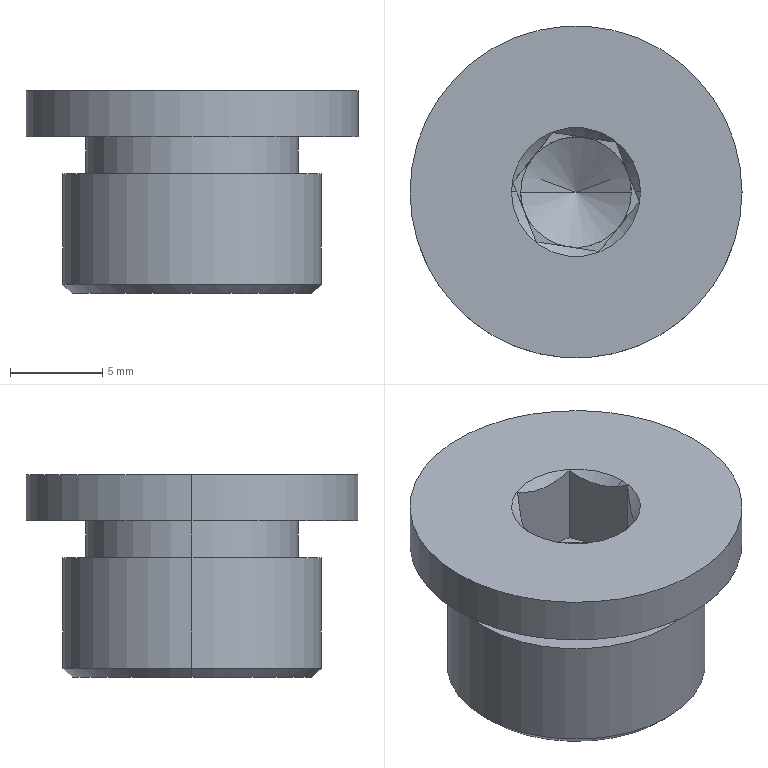Part | SolidWorks | features BaseBody 1 | 1 solid | 30 faces | box 18 x 18 x 11 mm | volume 1653 mm3 | plane 16 | cylinder 8 | cone 6 | commonest cylinder face diameters 6 x2 11.5 x2 14 x2 18 x2
STEP:
#1=CARTESIAN_POINT('',(-10.901,8.92,75.5));
#2=VERTEX_POINT('',#1);
#3=CARTESIAN_POINT('',(-28.901,8.92,75.5));
#4=VERTEX_POINT('',#3);
#5=CARTESIAN_POINT('',(-19.901,8.92,75.5));
#6=DIRECTION('',(0.,0.,1.));
#7=DIRECTION('',(1.,0.,0.));
#8=AXIS2_PLACEMENT_3D('',#5,#6,#7);
#9=CIRCLE('',#8,9.);
#10=EDGE_CURVE('',#2,#4,#9,.T.);
#11=ORIENTED_EDGE('',*,*,#10,.T.);
#12=CARTESIAN_POINT('',(-28.901,8.92,78.));
#13=VERTEX_POINT('',#12);
#14=CARTESIAN_POINT('',(-28.901,8.92,75.5));
#15=DIRECTION('',(0.,0.,1.));
#16=VECTOR('',#15,1000.);
#17=LINE('',#14,#16);
#18=EDGE_CURVE('',#4,#13,#17,.T.);
#19=ORIENTED_EDGE('',*,*,#18,.T.);
#20=CARTESIAN_POINT('',(-10.901,8.92,78.));
#21=VERTEX_POINT('',#20);
#22=CARTESIAN_POINT('',(-19.901,8.92,78.));
#23=DIRECTION('',(0.,0.,1.));
#24=DIRECTION('',(1.,0.,0.));
#25=AXIS2_PLACEMENT_3D('',#22,#23,#24);
#26=CIRCLE('',#25,9.);
#27=EDGE_CURVE('',#21,#13,#26,.T.);
#28=ORIENTED_EDGE('',*,*,#27,.F.);
#29=CARTESIAN_POINT('',(-10.901,8.92,75.5));
#30=DIRECTION('',(0.,0.,1.));
#31=VECTOR('',#30,1000.);
#32=LINE('',#29,#31);
#33=EDGE_CURVE('',#2,#21,#32,.T.);
#34=ORIENTED_EDGE('',*,*,#33,.F.);
#35=EDGE_LOOP('',(#11,#19,#28,#34));
#36=FACE_OUTER_BOUND('',#35,.T.);
#37=CARTESIAN_POINT('',(-19.901,8.92,75.5));
#38=DIRECTION('',(0.,0.,1.));
#39=DIRECTION('',(1.,0.,0.));
#40=AXIS2_PLACEMENT_3D('',#37,#38,#39);
#41=CYLINDRICAL_SURFACE('',#40,9.);
#42=ADVANCED_FACE('',(#36),#41,.T.);
#43=CARTESIAN_POINT('',(-14.151,8.92,73.5));
#44=VERTEX_POINT('',#43);
#45=CARTESIAN_POINT('',(-25.651,8.92,73.5));
#46=VERTEX_POINT('',#45);
#47=CARTESIAN_POINT('',(-19.901,8.92,73.5));
#48=DIRECTION('',(0.,0.,1.));
#49=DIRECTION('',(1.,0.,0.));
#50=AXIS2_PLACEMENT_3D('',#47,#48,#49);
#51=CIRCLE('',#50,5.75);
#52=EDGE_CURVE('',#44,#46,#51,.T.);
#53=ORIENTED_EDGE('',*,*,#52,.T.);
#54=CARTESIAN_POINT('',(-25.651,8.92,75.5));
#55=VERTEX_POINT('',#54);
#56=CARTESIAN_POINT('',(-25.651,8.92,73.5));
#57=DIRECTION('',(0.,0.,1.));
#58=VECTOR('',#57,1000.);
#59=LINE('',#56,#58);
#60=EDGE_CURVE('',#46,#55,#59,.T.);
#61=ORIENTED_EDGE('',*,*,#60,.T.);
#62=CARTESIAN_POINT('',(-14.151,8.92,75.5));
#63=VERTEX_POINT('',#62);
#64=CARTESIAN_POINT('',(-19.901,8.92,75.5));
#65=DIRECTION('',(0.,0.,-1.));
#66=DIRECTION('',(1.,0.,0.));
#67=AXIS2_PLACEMENT_3D('',#64,#65,#66);
#68=CIRCLE('',#67,5.75);
#69=EDGE_CURVE('',#55,#63,#68,.T.);
#70=ORIENTED_EDGE('',*,*,#69,.T.);
#71=CARTESIAN_POINT('',(-14.151,8.92,73.5));
#72=DIRECTION('',(0.,0.,1.));
#73=VECTOR('',#72,1000.);
#74=LINE('',#71,#73);
#75=EDGE_CURVE('',#44,#63,#74,.T.);
#76=ORIENTED_EDGE('',*,*,#75,.F.);
#77=EDGE_LOOP('',(#53,#61,#70,#76));
#78=FACE_OUTER_BOUND('',#77,.T.);
#79=CARTESIAN_POINT('',(-19.901,8.92,73.5));
#80=DIRECTION('',(0.,0.,1.));
#81=DIRECTION('',(1.,0.,0.));
#82=AXIS2_PLACEMENT_3D('',#79,#80,#81);
#83=CYLINDRICAL_SURFACE('',#82,5.75);
#84=ADVANCED_FACE('',(#78),#83,.T.);
#85=CARTESIAN_POINT('',(-22.901,8.92,72.5));
#86=VERTEX_POINT('',#85);
#87=CARTESIAN_POINT('',(-16.901,8.92,72.5));
#88=VERTEX_POINT('',#87);
#89=CARTESIAN_POINT('',(-19.901,8.92,72.5));
#90=DIRECTION('',(0.,0.,1.));
#91=DIRECTION('',(1.,0.,0.));
#92=AXIS2_PLACEMENT_3D('',#89,#90,#91);
#93=CIRCLE('',#92,3.);
#94=EDGE_CURVE('',#86,#88,#93,.T.);
#95=ORIENTED_EDGE('',*,*,#94,.F.);
#96=CARTESIAN_POINT('',(-22.901,8.92,73.5));
#97=VERTEX_POINT('',#96);
#98=CARTESIAN_POINT('',(-22.901,8.92,72.5));
#99=DIRECTION('',(0.,0.,1.));
#100=VECTOR('',#99,1000.);
#101=LINE('',#98,#100);
#102=EDGE_CURVE('',#86,#97,#101,.T.);
#103=ORIENTED_EDGE('',*,*,#102,.T.);
#104=CARTESIAN_POINT('',(-22.698,7.835,73.5));
#105=VERTEX_POINT('',#104);
#106=CARTESIAN_POINT('',(-19.901,8.92,73.5));
#107=DIRECTION('',(0.,0.,-1.));
#108=DIRECTION('',(1.,0.,0.));
#109=AXIS2_PLACEMENT_3D('',#106,#107,#108);
#110=CIRCLE('',#109,3.);
#111=EDGE_CURVE('',#105,#97,#110,.T.);
#112=ORIENTED_EDGE('',*,*,#111,.F.);
#113=CARTESIAN_POINT('',(-20.36,5.955,73.5));
#114=VERTEX_POINT('',#113);
#115=CARTESIAN_POINT('',(-19.901,8.92,73.5));
#116=DIRECTION('',(0.,0.,-1.));
#117=DIRECTION('',(1.,0.,0.));
#118=AXIS2_PLACEMENT_3D('',#115,#116,#117);
#119=CIRCLE('',#118,3.);
#120=EDGE_CURVE('',#114,#105,#119,.T.);
#121=ORIENTED_EDGE('',*,*,#120,.F.);
#122=CARTESIAN_POINT('',(-17.563,7.04,73.5));
#123=VERTEX_POINT('',#122);
#124=CARTESIAN_POINT('',(-19.901,8.92,73.5));
#125=DIRECTION('',(0.,0.,-1.));
#126=DIRECTION('',(1.,0.,0.));
#127=AXIS2_PLACEMENT_3D('',#124,#125,#126);
#128=CIRCLE('',#127,3.);
#129=EDGE_CURVE('',#123,#114,#128,.T.);
#130=ORIENTED_EDGE('',*,*,#129,.F.);
#131=CARTESIAN_POINT('',(-16.901,8.92,73.5));
#132=VERTEX_POINT('',#131);
#133=CARTESIAN_POINT('',(-19.901,8.92,73.5));
#134=DIRECTION('',(0.,0.,-1.));
#135=DIRECTION('',(1.,0.,0.));
#136=AXIS2_PLACEMENT_3D('',#133,#134,#135);
#137=CIRCLE('',#136,3.);
#138=EDGE_CURVE('',#132,#123,#137,.T.);
#139=ORIENTED_EDGE('',*,*,#138,.F.);
#140=CARTESIAN_POINT('',(-16.901,8.92,72.5));
#141=DIRECTION('',(0.,0.,1.));
#142=VECTOR('',#141,1000.);
#143=LINE('',#140,#142);
#144=EDGE_CURVE('',#88,#132,#143,.T.);
#145=ORIENTED_EDGE('',*,*,#144,.F.);
#146=EDGE_LOOP('',(#95,#103,#112,#121,#130,#139,#145));
#147=FACE_OUTER_BOUND('',#146,.T.);
#148=CARTESIAN_POINT('',(-19.901,8.92,72.5));
#149=DIRECTION('',(0.,0.,1.));
#150=DIRECTION('',(1.,0.,0.));
#151=AXIS2_PLACEMENT_3D('',#148,#149,#150);
#152=CYLINDRICAL_SURFACE('',#151,3.);
#153=ADVANCED_FACE('',(#147),#152,.F.);
#154=CARTESIAN_POINT('',(-19.901,8.92,70.768));
#155=VERTEX_POINT('',#154);
#156=CARTESIAN_POINT('',(-16.901,8.92,72.5));
#157=DIRECTION('',(0.866,0.,0.5));
#158=VECTOR('',#157,1000.);
#159=LINE('',#156,#158);
#160=EDGE_CURVE('',#155,#88,#159,.T.);
#161=ORIENTED_EDGE('',*,*,#160,.F.);
#162=CARTESIAN_POINT('',(-22.901,8.92,72.5));
#163=DIRECTION('',(-0.866,0.,0.5));
#164=VECTOR('',#163,1000.);
#165=LINE('',#162,#164);
#166=EDGE_CURVE('',#155,#86,#165,.T.);
#167=ORIENTED_EDGE('',*,*,#166,.T.);
#168=ORIENTED_EDGE('',*,*,#94,.T.);
#169=EDGE_LOOP('',(#161,#167,#168));
#170=FACE_OUTER_BOUND('',#169,.T.);
#171=CARTESIAN_POINT('',(-19.901,8.92,72.5));
#172=DIRECTION('',(0.,0.,1.));
#173=DIRECTION('',(1.,0.,0.));
#174=AXIS2_PLACEMENT_3D('',#171,#172,#173);
#175=CONICAL_SURFACE('',#174,3.,1.047);
#176=ADVANCED_FACE('',(#170),#175,.F.);
#177=CARTESIAN_POINT('',(-12.901,8.92,67.5));
#178=VERTEX_POINT('',#177);
#179=CARTESIAN_POINT('',(-26.901,8.92,67.5));
#180=VERTEX_POINT('',#179);
#181=CARTESIAN_POINT('',(-19.901,8.92,67.5));
#182=DIRECTION('',(0.,0.,1.));
#183=DIRECTION('',(1.,0.,0.));
#184=AXIS2_PLACEMENT_3D('',#181,#182,#183);
#185=CIRCLE('',#184,7.);
#186=EDGE_CURVE('',#178,#180,#185,.T.);
#187=ORIENTED_EDGE('',*,*,#186,.T.);
#188=CARTESIAN_POINT('',(-26.901,8.92,73.5));
#189=VERTEX_POINT('',#188);
#190=CARTESIAN_POINT('',(-26.901,8.92,67.5));
#191=DIRECTION('',(0.,0.,1.));
#192=VECTOR('',#191,1000.);
#193=LINE('',#190,#192);
#194=EDGE_CURVE('',#180,#189,#193,.T.);
#195=ORIENTED_EDGE('',*,*,#194,.T.);
#196=CARTESIAN_POINT('',(-12.901,8.92,73.5));
#197=VERTEX_POINT('',#196);
#198=CARTESIAN_POINT('',(-19.901,8.92,73.5));
#199=DIRECTION('',(0.,0.,1.));
#200=DIRECTION('',(1.,0.,0.));
#201=AXIS2_PLACEMENT_3D('',#198,#199,#200);
#202=CIRCLE('',#201,7.);
#203=EDGE_CURVE('',#197,#189,#202,.T.);
#204=ORIENTED_EDGE('',*,*,#203,.F.);
#205=CARTESIAN_POINT('',(-12.901,8.92,67.5));
#206=DIRECTION('',(0.,0.,1.));
#207=VECTOR('',#206,1000.);
#208=LINE('',#205,#207);
#209=EDGE_CURVE('',#178,#197,#208,.T.);
#210=ORIENTED_EDGE('',*,*,#209,.F.);
#211=EDGE_LOOP('',(#187,#195,#204,#210));
#212=FACE_OUTER_BOUND('',#211,.T.);
#213=CARTESIAN_POINT('',(-19.901,8.92,67.5));
#214=DIRECTION('',(0.,0.,1.));
#215=DIRECTION('',(1.,0.,0.));
#216=AXIS2_PLACEMENT_3D('',#213,#214,#215);
#217=CYLINDRICAL_SURFACE('',#216,7.);
#218=ADVANCED_FACE('',(#212),#217,.T.);
#219=CARTESIAN_POINT('',(-13.401,8.92,67.));
#220=VERTEX_POINT('',#219);
#221=CARTESIAN_POINT('',(-26.401,8.92,67.));
#222=VERTEX_POINT('',#221);
#223=CARTESIAN_POINT('',(-19.901,8.92,67.));
#224=DIRECTION('',(0.,0.,1.));
#225=DIRECTION('',(1.,0.,0.));
#226=AXIS2_PLACEMENT_3D('',#223,#224,#225);
#227=CIRCLE('',#226,6.5);
#228=EDGE_CURVE('',#220,#222,#227,.T.);
#229=ORIENTED_EDGE('',*,*,#228,.T.);
#230=CARTESIAN_POINT('',(-26.901,8.92,67.5));
#231=DIRECTION('',(-0.7071,0.,0.7071));
#232=VECTOR('',#231,1000.);
#233=LINE('',#230,#232);
#234=EDGE_CURVE('',#222,#180,#233,.T.);
#235=ORIENTED_EDGE('',*,*,#234,.T.);
#236=ORIENTED_EDGE('',*,*,#186,.F.);
#237=CARTESIAN_POINT('',(-12.901,8.92,67.5));
#238=DIRECTION('',(0.7071,0.,0.7071));
#239=VECTOR('',#238,1000.);
#240=LINE('',#237,#239);
#241=EDGE_CURVE('',#220,#178,#240,.T.);
#242=ORIENTED_EDGE('',*,*,#241,.F.);
#243=EDGE_LOOP('',(#229,#235,#236,#242));
#244=FACE_OUTER_BOUND('',#243,.T.);
#245=CARTESIAN_POINT('',(-19.901,8.92,67.5));
#246=DIRECTION('',(0.,0.,1.));
#247=DIRECTION('',(1.,0.,0.));
#248=AXIS2_PLACEMENT_3D('',#245,#246,#247);
#249=CONICAL_SURFACE('',#248,7.,0.7854);
#250=ADVANCED_FACE('',(#244),#249,.T.);
#251=CARTESIAN_POINT('',(-16.401,8.92,78.));
#252=VERTEX_POINT('',#251);
#253=CARTESIAN_POINT('',(-23.401,8.92,78.));
#254=VERTEX_POINT('',#253);
#255=CARTESIAN_POINT('',(-19.901,8.92,78.));
#256=DIRECTION('',(0.,0.,-1.));
#257=DIRECTION('',(1.,0.,0.));
#258=AXIS2_PLACEMENT_3D('',#255,#256,#257);
#259=CIRCLE('',#258,3.5);
#260=EDGE_CURVE('',#252,#254,#259,.T.);
#261=ORIENTED_EDGE('',*,*,#260,.T.);
#262=CARTESIAN_POINT('',(-19.901,8.92,78.));
#263=DIRECTION('',(0.,0.,-1.));
#264=DIRECTION('',(1.,0.,0.));
#265=AXIS2_PLACEMENT_3D('',#262,#263,#264);
#266=CIRCLE('',#265,3.5);
#267=EDGE_CURVE('',#254,#252,#266,.T.);
#268=ORIENTED_EDGE('',*,*,#267,.T.);
#269=EDGE_LOOP('',(#261,#268));
#270=FACE_BOUND('',#269,.T.);
#271=ORIENTED_EDGE('',*,*,#27,.T.);
#272=CARTESIAN_POINT('',(-19.901,8.92,78.));
#273=DIRECTION('',(0.,0.,1.));
#274=DIRECTION('',(1.,0.,0.));
#275=AXIS2_PLACEMENT_3D('',#272,#273,#274);
#276=CIRCLE('',#275,9.);
#277=EDGE_CURVE('',#13,#21,#276,.T.);
#278=ORIENTED_EDGE('',*,*,#277,.T.);
#279=EDGE_LOOP('',(#271,#278));
#280=FACE_OUTER_BOUND('',#279,.T.);
#281=CARTESIAN_POINT('',(-19.901,8.92,78.));
#282=DIRECTION('',(0.,0.,1.));
#283=DIRECTION('',(1.,0.,0.));
#284=AXIS2_PLACEMENT_3D('',#281,#282,#283);
#285=PLANE('',#284);
#286=ADVANCED_FACE('',(#270,#280),#285,.T.);
#287=CARTESIAN_POINT('',(-23.325,9.449,77.964));
#288=VERTEX_POINT('',#287);
#289=CARTESIAN_POINT('',(-23.119,8.92,77.718));
#290=VERTEX_POINT('',#289);
#291=CARTESIAN_POINT('',(-23.325,9.449,77.964));
#292=CARTESIAN_POINT('',(-23.258,9.277,77.872));
#293=CARTESIAN_POINT('',(-23.189,9.101,77.788));
#294=CARTESIAN_POINT('',(-23.119,8.92,77.718));
#295=B_SPLINE_CURVE_WITH_KNOTS('',3,(#291,#292,#293,#294),.UNSPECIFIED.,.F.,.F.,(4,4),(0.,0.0006191),.UNSPECIFIED.);
#296=EDGE_CURVE('',#288,#290,#295,.T.);
#297=ORIENTED_EDGE('',*,*,#296,.F.);
#298=CARTESIAN_POINT('',(-21.154,12.149,77.964));
#299=VERTEX_POINT('',#298);
#300=CARTESIAN_POINT('',(-21.154,12.149,77.964));
#301=CARTESIAN_POINT('',(-21.324,11.938,77.829));
#302=CARTESIAN_POINT('',(-21.497,11.723,77.714));
#303=CARTESIAN_POINT('',(-21.767,11.388,77.59));
#304=CARTESIAN_POINT('',(-21.858,11.274,77.558));
#305=CARTESIAN_POINT('',(-22.045,11.042,77.512));
#306=CARTESIAN_POINT('',(-22.141,10.922,77.5));
#307=CARTESIAN_POINT('',(-22.425,10.569,77.499));
#308=CARTESIAN_POINT('',(-22.611,10.337,77.545));
#309=CARTESIAN_POINT('',(-22.978,9.88,77.711));
#310=CARTESIAN_POINT('',(-23.154,9.662,77.828));
#311=CARTESIAN_POINT('',(-23.325,9.449,77.964));
#312=B_SPLINE_CURVE_WITH_KNOTS('',3,(#300,#301,#302,#303,#304,#305,#306,#307,#308,#309,#310,#311),.UNSPECIFIED.,.F.,.F.,(4,2,2,2,2,4),(0.,0.0008946,0.001342,0.001789,0.002684,0.003578),.UNSPECIFIED.);
#313=EDGE_CURVE('',#299,#288,#312,.T.);
#314=ORIENTED_EDGE('',*,*,#313,.F.);
#315=CARTESIAN_POINT('',(-17.731,11.62,77.964));
#316=VERTEX_POINT('',#315);
#317=CARTESIAN_POINT('',(-17.731,11.62,77.964));
#318=CARTESIAN_POINT('',(-17.998,11.661,77.829));
#319=CARTESIAN_POINT('',(-18.272,11.703,77.714));
#320=CARTESIAN_POINT('',(-18.697,11.769,77.59));
#321=CARTESIAN_POINT('',(-18.841,11.791,77.558));
#322=CARTESIAN_POINT('',(-19.135,11.837,77.512));
#323=CARTESIAN_POINT('',(-19.287,11.86,77.5));
#324=CARTESIAN_POINT('',(-19.735,11.93,77.499));
#325=CARTESIAN_POINT('',(-20.029,11.975,77.545));
#326=CARTESIAN_POINT('',(-20.608,12.065,77.711));
#327=CARTESIAN_POINT('',(-20.885,12.108,77.828));
#328=CARTESIAN_POINT('',(-21.154,12.149,77.964));
#329=B_SPLINE_CURVE_WITH_KNOTS('',3,(#317,#318,#319,#320,#321,#322,#323,#324,#325,#326,#327,#328),.UNSPECIFIED.,.F.,.F.,(4,2,2,2,2,4),(0.,0.0008946,0.001342,0.001789,0.002684,0.003578),.UNSPECIFIED.);
#330=EDGE_CURVE('',#316,#299,#329,.T.);
#331=ORIENTED_EDGE('',*,*,#330,.F.);
#332=CARTESIAN_POINT('',(-16.683,8.92,77.718));
#333=VERTEX_POINT('',#332);
#334=CARTESIAN_POINT('',(-16.683,8.92,77.718));
#335=CARTESIAN_POINT('',(-16.769,9.14,77.632));
#336=CARTESIAN_POINT('',(-16.856,9.365,77.568));
#337=CARTESIAN_POINT('',(-17.034,9.823,77.496));
#338=CARTESIAN_POINT('',(-17.126,10.061,77.49));
#339=CARTESIAN_POINT('',(-17.395,10.755,77.566));
#340=CARTESIAN_POINT('',(-17.568,11.2,77.739));
#341=CARTESIAN_POINT('',(-17.731,11.62,77.964));
#342=B_SPLINE_CURVE_WITH_KNOTS('',3,(#334,#335,#336,#337,#338,#339,#340,#341),.UNSPECIFIED.,.F.,.F.,(4,2,2,4),(0.,0.0007448,0.00149,0.002979),.UNSPECIFIED.);
#343=EDGE_CURVE('',#333,#316,#342,.T.);
#344=ORIENTED_EDGE('',*,*,#343,.F.);
#345=CARTESIAN_POINT('',(-16.401,8.92,78.));
#346=CARTESIAN_POINT('',(-16.683,8.92,77.718));
#347=B_SPLINE_CURVE_WITH_KNOTS('',1,(#345,#346),.UNSPECIFIED.,.F.,.F.,(2,2),(0.,1.),.UNSPECIFIED.);
#348=EDGE_CURVE('',#252,#333,#347,.T.);
#349=ORIENTED_EDGE('',*,*,#348,.F.);
#350=ORIENTED_EDGE('',*,*,#267,.F.);
#351=CARTESIAN_POINT('',(-23.119,8.92,77.718));
#352=CARTESIAN_POINT('',(-23.401,8.92,78.));
#353=B_SPLINE_CURVE_WITH_KNOTS('',1,(#351,#352),.UNSPECIFIED.,.F.,.F.,(2,2),(0.,1.),.UNSPECIFIED.);
#354=EDGE_CURVE('',#290,#254,#353,.T.);
#355=ORIENTED_EDGE('',*,*,#354,.F.);
#356=EDGE_LOOP('',(#297,#314,#331,#344,#349,#350,#355));
#357=FACE_OUTER_BOUND('',#356,.T.);
#358=CARTESIAN_POINT('',(-19.901,8.92,78.));
#359=DIRECTION('',(0.,0.,1.));
#360=DIRECTION('',(1.,0.,0.));
#361=AXIS2_PLACEMENT_3D('',#358,#359,#360);
#362=CONICAL_SURFACE('',#361,3.5,0.7854);
#363=ADVANCED_FACE('',(#357),#362,.F.);
#364=ORIENTED_EDGE('',*,*,#354,.T.);
#365=ORIENTED_EDGE('',*,*,#260,.F.);
#366=ORIENTED_EDGE('',*,*,#348,.T.);
#367=CARTESIAN_POINT('',(-16.478,8.39,77.964));
#368=VERTEX_POINT('',#367);
#369=CARTESIAN_POINT('',(-16.478,8.39,77.964));
#370=CARTESIAN_POINT('',(-16.545,8.563,77.872));
#371=CARTESIAN_POINT('',(-16.613,8.739,77.788));
#372=CARTESIAN_POINT('',(-16.683,8.92,77.718));
#373=B_SPLINE_CURVE_WITH_KNOTS('',3,(#369,#370,#371,#372),.UNSPECIFIED.,.F.,.F.,(4,4),(0.,0.0006191),.UNSPECIFIED.);
#374=EDGE_CURVE('',#368,#333,#373,.T.);
#375=ORIENTED_EDGE('',*,*,#374,.F.);
#376=CARTESIAN_POINT('',(-18.648,5.69,77.964));
#377=VERTEX_POINT('',#376);
#378=CARTESIAN_POINT('',(-18.648,5.69,77.964));
#379=CARTESIAN_POINT('',(-18.479,5.901,77.829));
#380=CARTESIAN_POINT('',(-18.305,6.117,77.714));
#381=CARTESIAN_POINT('',(-18.036,6.452,77.59));
#382=CARTESIAN_POINT('',(-17.944,6.566,77.558));
#383=CARTESIAN_POINT('',(-17.758,6.798,77.512));
#384=CARTESIAN_POINT('',(-17.662,6.917,77.5));
#385=CARTESIAN_POINT('',(-17.378,7.271,77.499));
#386=CARTESIAN_POINT('',(-17.191,7.503,77.545));
#387=CARTESIAN_POINT('',(-16.824,7.96,77.711));
#388=CARTESIAN_POINT('',(-16.648,8.178,77.828));
#389=CARTESIAN_POINT('',(-16.478,8.39,77.964));
#390=B_SPLINE_CURVE_WITH_KNOTS('',3,(#378,#379,#380,#381,#382,#383,#384,#385,#386,#387,#388,#389),.UNSPECIFIED.,.F.,.F.,(4,2,2,2,2,4),(0.,0.0008946,0.001342,0.001789,0.002684,0.003578),.UNSPECIFIED.);
#391=EDGE_CURVE('',#377,#368,#390,.T.);
#392=ORIENTED_EDGE('',*,*,#391,.F.);
#393=CARTESIAN_POINT('',(-22.072,6.22,77.964));
#394=VERTEX_POINT('',#393);
#395=CARTESIAN_POINT('',(-22.072,6.22,77.964));
#396=CARTESIAN_POINT('',(-21.804,6.179,77.829));
#397=CARTESIAN_POINT('',(-21.531,6.136,77.714));
#398=CARTESIAN_POINT('',(-21.106,6.07,77.59));
#399=CARTESIAN_POINT('',(-20.962,6.048,77.558));
#400=CARTESIAN_POINT('',(-20.667,6.003,77.512));
#401=CARTESIAN_POINT('',(-20.516,5.979,77.5));
#402=CARTESIAN_POINT('',(-20.067,5.91,77.499));
#403=CARTESIAN_POINT('',(-19.774,5.864,77.545));
#404=CARTESIAN_POINT('',(-19.194,5.775,77.711));
#405=CARTESIAN_POINT('',(-18.917,5.732,77.828));
#406=CARTESIAN_POINT('',(-18.648,5.69,77.964));
#407=B_SPLINE_CURVE_WITH_KNOTS('',3,(#395,#396,#397,#398,#399,#400,#401,#402,#403,#404,#405,#406),.UNSPECIFIED.,.F.,.F.,(4,2,2,2,2,4),(0.,0.0008946,0.001342,0.001789,0.002684,0.003578),.UNSPECIFIED.);
#408=EDGE_CURVE('',#394,#377,#407,.T.);
#409=ORIENTED_EDGE('',*,*,#408,.F.);
#410=CARTESIAN_POINT('',(-23.119,8.92,77.718));
#411=CARTESIAN_POINT('',(-23.034,8.699,77.632));
#412=CARTESIAN_POINT('',(-22.947,8.475,77.568));
#413=CARTESIAN_POINT('',(-22.769,8.017,77.496));
#414=CARTESIAN_POINT('',(-22.676,7.779,77.49));
#415=CARTESIAN_POINT('',(-22.407,7.085,77.566));
#416=CARTESIAN_POINT('',(-22.234,6.639,77.739));
#417=CARTESIAN_POINT('',(-22.072,6.22,77.964));
#418=B_SPLINE_CURVE_WITH_KNOTS('',3,(#410,#411,#412,#413,#414,#415,#416,#417),.UNSPECIFIED.,.F.,.F.,(4,2,2,4),(0.,0.0007448,0.00149,0.002979),.UNSPECIFIED.);
#419=EDGE_CURVE('',#290,#394,#418,.T.);
#420=ORIENTED_EDGE('',*,*,#419,.F.);
#421=EDGE_LOOP('',(#364,#365,#366,#375,#392,#409,#420));
#422=FACE_OUTER_BOUND('',#421,.T.);
#423=CARTESIAN_POINT('',(-19.901,8.92,78.));
#424=DIRECTION('',(0.,0.,1.));
#425=DIRECTION('',(1.,0.,0.));
#426=AXIS2_PLACEMENT_3D('',#423,#424,#425);
#427=CONICAL_SURFACE('',#426,3.5,0.7854);
#428=ADVANCED_FACE('',(#422),#427,.F.);
#429=ORIENTED_EDGE('',*,*,#18,.F.);
#430=CARTESIAN_POINT('',(-19.901,8.92,75.5));
#431=DIRECTION('',(0.,0.,1.));
#432=DIRECTION('',(1.,0.,0.));
#433=AXIS2_PLACEMENT_3D('',#430,#431,#432);
#434=CIRCLE('',#433,9.);
#435=EDGE_CURVE('',#4,#2,#434,.T.);
#436=ORIENTED_EDGE('',*,*,#435,.T.);
#437=ORIENTED_EDGE('',*,*,#33,.T.);
#438=ORIENTED_EDGE('',*,*,#277,.F.);
#439=EDGE_LOOP('',(#429,#436,#437,#438));
#440=FACE_OUTER_BOUND('',#439,.T.);
#441=CARTESIAN_POINT('',(-19.901,8.92,75.5));
#442=DIRECTION('',(0.,0.,1.));
#443=DIRECTION('',(1.,0.,0.));
#444=AXIS2_PLACEMENT_3D('',#441,#442,#443);
#445=CYLINDRICAL_SURFACE('',#444,9.);
#446=ADVANCED_FACE('',(#440),#445,.T.);
#447=ORIENTED_EDGE('',*,*,#313,.T.);
#448=CARTESIAN_POINT('',(-23.325,9.449,73.5));
#449=VERTEX_POINT('',#448);
#450=CARTESIAN_POINT('',(-23.325,9.449,75.732));
#451=DIRECTION('',(0.,0.,-1.));
#452=VECTOR('',#451,1000.);
#453=LINE('',#450,#452);
#454=EDGE_CURVE('',#288,#449,#453,.T.);
#455=ORIENTED_EDGE('',*,*,#454,.T.);
#456=CARTESIAN_POINT('',(-22.239,10.799,73.5));
#457=VERTEX_POINT('',#456);
#458=CARTESIAN_POINT('',(-22.239,10.799,73.5));
#459=DIRECTION('',(-0.6265,-0.7794,0.));
#460=VECTOR('',#459,1000.);
#461=LINE('',#458,#460);
#462=EDGE_CURVE('',#457,#449,#461,.T.);
#463=ORIENTED_EDGE('',*,*,#462,.F.);
#464=CARTESIAN_POINT('',(-21.154,12.149,73.5));
#465=VERTEX_POINT('',#464);
#466=CARTESIAN_POINT('',(-21.154,12.149,73.5));
#467=DIRECTION('',(-0.6265,-0.7794,0.));
#468=VECTOR('',#467,1000.);
#469=LINE('',#466,#468);
#470=EDGE_CURVE('',#465,#457,#469,.T.);
#471=ORIENTED_EDGE('',*,*,#470,.F.);
#472=CARTESIAN_POINT('',(-21.154,12.149,75.732));
#473=DIRECTION('',(0.,0.,1.));
#474=VECTOR('',#473,1000.);
#475=LINE('',#472,#474);
#476=EDGE_CURVE('',#465,#299,#475,.T.);
#477=ORIENTED_EDGE('',*,*,#476,.T.);
#478=EDGE_LOOP('',(#447,#455,#463,#471,#477));
#479=FACE_OUTER_BOUND('',#478,.T.);
#480=CARTESIAN_POINT('',(-22.239,10.799,75.732));
#481=DIRECTION('',(0.7794,-0.6265,0.));
#482=DIRECTION('',(0.6265,0.7794,0.));
#483=AXIS2_PLACEMENT_3D('',#480,#481,#482);
#484=PLANE('',#483);
#485=ADVANCED_FACE('',(#479),#484,.T.);
#486=CARTESIAN_POINT('',(-17.731,11.62,73.5));
#487=VERTEX_POINT('',#486);
#488=CARTESIAN_POINT('',(-19.443,11.885,73.5));
#489=VERTEX_POINT('',#488);
#490=CARTESIAN_POINT('',(-17.731,11.62,73.5));
#491=DIRECTION('',(-0.9882,0.1529,0.));
#492=VECTOR('',#491,1000.);
#493=LINE('',#490,#492);
#494=EDGE_CURVE('',#487,#489,#493,.T.);
#495=ORIENTED_EDGE('',*,*,#494,.F.);
#496=CARTESIAN_POINT('',(-17.731,11.62,75.732));
#497=DIRECTION('',(0.,0.,-1.));
#498=VECTOR('',#497,1000.);
#499=LINE('',#496,#498);
#500=EDGE_CURVE('',#316,#487,#499,.T.);
#501=ORIENTED_EDGE('',*,*,#500,.F.);
#502=ORIENTED_EDGE('',*,*,#330,.T.);
#503=ORIENTED_EDGE('',*,*,#476,.F.);
#504=CARTESIAN_POINT('',(-19.443,11.885,73.5));
#505=DIRECTION('',(-0.9882,0.1529,0.));
#506=VECTOR('',#505,1000.);
#507=LINE('',#504,#506);
#508=EDGE_CURVE('',#489,#465,#507,.T.);
#509=ORIENTED_EDGE('',*,*,#508,.F.);
#510=EDGE_LOOP('',(#495,#501,#502,#503,#509));
#511=FACE_OUTER_BOUND('',#510,.T.);
#512=CARTESIAN_POINT('',(-19.443,11.885,75.732));
#513=DIRECTION('',(0.1529,0.9882,0.));
#514=DIRECTION('',(-0.9882,0.1529,0.));
#515=AXIS2_PLACEMENT_3D('',#512,#513,#514);
#516=PLANE('',#515);
#517=ADVANCED_FACE('',(#511),#516,.F.);
#518=CARTESIAN_POINT('',(-16.478,8.39,73.5));
#519=VERTEX_POINT('',#518);
#520=CARTESIAN_POINT('',(-17.104,10.005,73.5));
#521=VERTEX_POINT('',#520);
#522=CARTESIAN_POINT('',(-16.478,8.39,73.5));
#523=DIRECTION('',(-0.3617,0.9323,0.));
#524=VECTOR('',#523,1000.);
#525=LINE('',#522,#524);
#526=EDGE_CURVE('',#519,#521,#525,.T.);
#527=ORIENTED_EDGE('',*,*,#526,.F.);
#528=CARTESIAN_POINT('',(-16.478,8.39,75.732));
#529=DIRECTION('',(0.,0.,-1.));
#530=VECTOR('',#529,1000.);
#531=LINE('',#528,#530);
#532=EDGE_CURVE('',#368,#519,#531,.T.);
#533=ORIENTED_EDGE('',*,*,#532,.F.);
#534=ORIENTED_EDGE('',*,*,#374,.T.);
#535=ORIENTED_EDGE('',*,*,#343,.T.);
#536=ORIENTED_EDGE('',*,*,#500,.T.);
#537=CARTESIAN_POINT('',(-17.104,10.005,73.5));
#538=DIRECTION('',(-0.3617,0.9323,0.));
#539=VECTOR('',#538,1000.);
#540=LINE('',#537,#539);
#541=EDGE_CURVE('',#521,#487,#540,.T.);
#542=ORIENTED_EDGE('',*,*,#541,.F.);
#543=EDGE_LOOP('',(#527,#533,#534,#535,#536,#542));
#544=FACE_OUTER_BOUND('',#543,.T.);
#545=CARTESIAN_POINT('',(-17.104,10.005,75.732));
#546=DIRECTION('',(0.9323,0.3617,0.));
#547=DIRECTION('',(-0.3617,0.9323,0.));
#548=AXIS2_PLACEMENT_3D('',#545,#546,#547);
#549=PLANE('',#548);
#550=ADVANCED_FACE('',(#544),#549,.F.);
#551=ORIENTED_EDGE('',*,*,#419,.T.);
#552=CARTESIAN_POINT('',(-22.072,6.22,73.5));
#553=VERTEX_POINT('',#552);
#554=CARTESIAN_POINT('',(-22.072,6.22,75.732));
#555=DIRECTION('',(0.,0.,-1.));
#556=VECTOR('',#555,1000.);
#557=LINE('',#554,#556);
#558=EDGE_CURVE('',#394,#553,#557,.T.);
#559=ORIENTED_EDGE('',*,*,#558,.T.);
#560=CARTESIAN_POINT('',(-22.698,7.835,73.5));
#561=DIRECTION('',(0.3617,-0.9323,0.));
#562=VECTOR('',#561,1000.);
#563=LINE('',#560,#562);
#564=EDGE_CURVE('',#105,#553,#563,.T.);
#565=ORIENTED_EDGE('',*,*,#564,.F.);
#566=CARTESIAN_POINT('',(-23.325,9.449,73.5));
#567=DIRECTION('',(0.3617,-0.9323,0.));
#568=VECTOR('',#567,1000.);
#569=LINE('',#566,#568);
#570=EDGE_CURVE('',#449,#105,#569,.T.);
#571=ORIENTED_EDGE('',*,*,#570,.F.);
#572=ORIENTED_EDGE('',*,*,#454,.F.);
#573=ORIENTED_EDGE('',*,*,#296,.T.);
#574=EDGE_LOOP('',(#551,#559,#565,#571,#572,#573));
#575=FACE_OUTER_BOUND('',#574,.T.);
#576=CARTESIAN_POINT('',(-22.698,7.835,75.732));
#577=DIRECTION('',(0.9323,0.3617,0.));
#578=DIRECTION('',(-0.3617,0.9323,0.));
#579=AXIS2_PLACEMENT_3D('',#576,#577,#578);
#580=PLANE('',#579);
#581=ADVANCED_FACE('',(#575),#580,.T.);
#582=CARTESIAN_POINT('',(-17.563,7.04,73.5));
#583=DIRECTION('',(0.6265,0.7794,0.));
#584=VECTOR('',#583,1000.);
#585=LINE('',#582,#584);
#586=EDGE_CURVE('',#123,#519,#585,.T.);
#587=ORIENTED_EDGE('',*,*,#586,.F.);
#588=CARTESIAN_POINT('',(-18.648,5.69,73.5));
#589=VERTEX_POINT('',#588);
#590=CARTESIAN_POINT('',(-18.648,5.69,73.5));
#591=DIRECTION('',(0.6265,0.7794,0.));
#592=VECTOR('',#591,1000.);
#593=LINE('',#590,#592);
#594=EDGE_CURVE('',#589,#123,#593,.T.);
#595=ORIENTED_EDGE('',*,*,#594,.F.);
#596=CARTESIAN_POINT('',(-18.648,5.69,75.732));
#597=DIRECTION('',(0.,0.,-1.));
#598=VECTOR('',#597,1000.);
#599=LINE('',#596,#598);
#600=EDGE_CURVE('',#377,#589,#599,.T.);
#601=ORIENTED_EDGE('',*,*,#600,.F.);
#602=ORIENTED_EDGE('',*,*,#391,.T.);
#603=ORIENTED_EDGE('',*,*,#532,.T.);
#604=EDGE_LOOP('',(#587,#595,#601,#602,#603));
#605=FACE_OUTER_BOUND('',#604,.T.);
#606=CARTESIAN_POINT('',(-17.563,7.04,75.732));
#607=DIRECTION('',(0.7794,-0.6265,0.));
#608=DIRECTION('',(0.6265,0.7794,0.));
#609=AXIS2_PLACEMENT_3D('',#606,#607,#608);
#610=PLANE('',#609);
#611=ADVANCED_FACE('',(#605),#610,.F.);
#612=ORIENTED_EDGE('',*,*,#408,.T.);
#613=ORIENTED_EDGE('',*,*,#600,.T.);
#614=CARTESIAN_POINT('',(-20.36,5.955,73.5));
#615=DIRECTION('',(0.9882,-0.1529,0.));
#616=VECTOR('',#615,1000.);
#617=LINE('',#614,#616);
#618=EDGE_CURVE('',#114,#589,#617,.T.);
#619=ORIENTED_EDGE('',*,*,#618,.F.);
#620=CARTESIAN_POINT('',(-20.36,5.955,73.5));
#621=DIRECTION('',(-0.9882,0.1529,0.));
#622=VECTOR('',#621,1000.);
#623=LINE('',#620,#622);
#624=EDGE_CURVE('',#114,#553,#623,.T.);
#625=ORIENTED_EDGE('',*,*,#624,.T.);
#626=ORIENTED_EDGE('',*,*,#558,.F.);
#627=EDGE_LOOP('',(#612,#613,#619,#625,#626));
#628=FACE_OUTER_BOUND('',#627,.T.);
#629=CARTESIAN_POINT('',(-20.36,5.955,75.732));
#630=DIRECTION('',(0.1529,0.9882,0.));
#631=DIRECTION('',(-0.9882,0.1529,0.));
#632=AXIS2_PLACEMENT_3D('',#629,#630,#631);
#633=PLANE('',#632);
#634=ADVANCED_FACE('',(#628),#633,.T.);
#635=CARTESIAN_POINT('',(-19.901,8.92,75.5));
#636=DIRECTION('',(0.,0.,-1.));
#637=DIRECTION('',(1.,0.,0.));
#638=AXIS2_PLACEMENT_3D('',#635,#636,#637);
#639=CIRCLE('',#638,5.75);
#640=EDGE_CURVE('',#63,#55,#639,.T.);
#641=ORIENTED_EDGE('',*,*,#640,.F.);
#642=ORIENTED_EDGE('',*,*,#69,.F.);
#643=EDGE_LOOP('',(#641,#642));
#644=FACE_BOUND('',#643,.T.);
#645=ORIENTED_EDGE('',*,*,#10,.F.);
#646=ORIENTED_EDGE('',*,*,#435,.F.);
#647=EDGE_LOOP('',(#645,#646));
#648=FACE_OUTER_BOUND('',#647,.T.);
#649=CARTESIAN_POINT('',(-19.901,8.92,75.5));
#650=DIRECTION('',(0.,0.,1.));
#651=DIRECTION('',(1.,0.,0.));
#652=AXIS2_PLACEMENT_3D('',#649,#650,#651);
#653=PLANE('',#652);
#654=ADVANCED_FACE('',(#644,#648),#653,.F.);
#655=ORIENTED_EDGE('',*,*,#624,.F.);
#656=ORIENTED_EDGE('',*,*,#120,.T.);
#657=ORIENTED_EDGE('',*,*,#564,.T.);
#658=EDGE_LOOP('',(#655,#656,#657));
#659=FACE_OUTER_BOUND('',#658,.T.);
#660=CARTESIAN_POINT('',(-21.529,6.895,73.5));
#661=DIRECTION('',(0.,0.,1.));
#662=DIRECTION('',(1.,0.,0.));
#663=AXIS2_PLACEMENT_3D('',#660,#661,#662);
#664=PLANE('',#663);
#665=ADVANCED_FACE('',(#659),#664,.T.);
#666=ORIENTED_EDGE('',*,*,#60,.F.);
#667=CARTESIAN_POINT('',(-19.901,8.92,73.5));
#668=DIRECTION('',(0.,0.,1.));
#669=DIRECTION('',(1.,0.,0.));
#670=AXIS2_PLACEMENT_3D('',#667,#668,#669);
#671=CIRCLE('',#670,5.75);
#672=EDGE_CURVE('',#46,#44,#671,.T.);
#673=ORIENTED_EDGE('',*,*,#672,.T.);
#674=ORIENTED_EDGE('',*,*,#75,.T.);
#675=ORIENTED_EDGE('',*,*,#640,.T.);
#676=EDGE_LOOP('',(#666,#673,#674,#675));
#677=FACE_OUTER_BOUND('',#676,.T.);
#678=CARTESIAN_POINT('',(-19.901,8.92,73.5));
#679=DIRECTION('',(0.,0.,1.));
#680=DIRECTION('',(1.,0.,0.));
#681=AXIS2_PLACEMENT_3D('',#678,#679,#680);
#682=CYLINDRICAL_SURFACE('',#681,5.75);
#683=ADVANCED_FACE('',(#677),#682,.T.);
#684=ORIENTED_EDGE('',*,*,#102,.F.);
#685=CARTESIAN_POINT('',(-19.901,8.92,72.5));
#686=DIRECTION('',(0.,0.,1.));
#687=DIRECTION('',(1.,0.,0.));
#688=AXIS2_PLACEMENT_3D('',#685,#686,#687);
#689=CIRCLE('',#688,3.);
#690=EDGE_CURVE('',#88,#86,#689,.T.);
#691=ORIENTED_EDGE('',*,*,#690,.F.);
#692=ORIENTED_EDGE('',*,*,#144,.T.);
#693=CARTESIAN_POINT('',(-19.901,8.92,73.5));
#694=DIRECTION('',(0.,0.,-1.));
#695=DIRECTION('',(1.,0.,0.));
#696=AXIS2_PLACEMENT_3D('',#693,#694,#695);
#697=CIRCLE('',#696,3.);
#698=EDGE_CURVE('',#521,#132,#697,.T.);
#699=ORIENTED_EDGE('',*,*,#698,.F.);
#700=CARTESIAN_POINT('',(-19.901,8.92,73.5));
#701=DIRECTION('',(0.,0.,-1.));
#702=DIRECTION('',(1.,0.,0.));
#703=AXIS2_PLACEMENT_3D('',#700,#701,#702);
#704=CIRCLE('',#703,3.);
#705=EDGE_CURVE('',#489,#521,#704,.T.);
#706=ORIENTED_EDGE('',*,*,#705,.F.);
#707=CARTESIAN_POINT('',(-19.901,8.92,73.5));
#708=DIRECTION('',(0.,0.,-1.));
#709=DIRECTION('',(1.,0.,0.));
#710=AXIS2_PLACEMENT_3D('',#707,#708,#709);
#711=CIRCLE('',#710,3.);
#712=EDGE_CURVE('',#457,#489,#711,.T.);
#713=ORIENTED_EDGE('',*,*,#712,.F.);
#714=CARTESIAN_POINT('',(-19.901,8.92,73.5));
#715=DIRECTION('',(0.,0.,-1.));
#716=DIRECTION('',(1.,0.,0.));
#717=AXIS2_PLACEMENT_3D('',#714,#715,#716);
#718=CIRCLE('',#717,3.);
#719=EDGE_CURVE('',#97,#457,#718,.T.);
#720=ORIENTED_EDGE('',*,*,#719,.F.);
#721=EDGE_LOOP('',(#684,#691,#692,#699,#706,#713,#720));
#722=FACE_OUTER_BOUND('',#721,.T.);
#723=CARTESIAN_POINT('',(-19.901,8.92,72.5));
#724=DIRECTION('',(0.,0.,1.));
#725=DIRECTION('',(1.,0.,0.));
#726=AXIS2_PLACEMENT_3D('',#723,#724,#725);
#727=CYLINDRICAL_SURFACE('',#726,3.);
#728=ADVANCED_FACE('',(#722),#727,.F.);
#729=ORIENTED_EDGE('',*,*,#52,.F.);
#730=ORIENTED_EDGE('',*,*,#672,.F.);
#731=EDGE_LOOP('',(#729,#730));
#732=FACE_BOUND('',#731,.T.);
#733=ORIENTED_EDGE('',*,*,#203,.T.);
#734=CARTESIAN_POINT('',(-19.901,8.92,73.5));
#735=DIRECTION('',(0.,0.,1.));
#736=DIRECTION('',(1.,0.,0.));
#737=AXIS2_PLACEMENT_3D('',#734,#735,#736);
#738=CIRCLE('',#737,7.);
#739=EDGE_CURVE('',#189,#197,#738,.T.);
#740=ORIENTED_EDGE('',*,*,#739,.T.);
#741=EDGE_LOOP('',(#733,#740));
#742=FACE_OUTER_BOUND('',#741,.T.);
#743=CARTESIAN_POINT('',(-19.901,8.92,73.5));
#744=DIRECTION('',(0.,0.,1.));
#745=DIRECTION('',(1.,0.,0.));
#746=AXIS2_PLACEMENT_3D('',#743,#744,#745);
#747=PLANE('',#746);
#748=ADVANCED_FACE('',(#732,#742),#747,.T.);
#749=ORIENTED_EDGE('',*,*,#166,.F.);
#750=ORIENTED_EDGE('',*,*,#160,.T.);
#751=ORIENTED_EDGE('',*,*,#690,.T.);
#752=EDGE_LOOP('',(#749,#750,#751));
#753=FACE_OUTER_BOUND('',#752,.T.);
#754=CARTESIAN_POINT('',(-19.901,8.92,72.5));
#755=DIRECTION('',(0.,0.,1.));
#756=DIRECTION('',(1.,0.,0.));
#757=AXIS2_PLACEMENT_3D('',#754,#755,#756);
#758=CONICAL_SURFACE('',#757,3.,1.047);
#759=ADVANCED_FACE('',(#753),#758,.F.);
#760=ORIENTED_EDGE('',*,*,#594,.T.);
#761=ORIENTED_EDGE('',*,*,#129,.T.);
#762=ORIENTED_EDGE('',*,*,#618,.T.);
#763=EDGE_LOOP('',(#760,#761,#762));
#764=FACE_OUTER_BOUND('',#763,.T.);
#765=CARTESIAN_POINT('',(-18.961,6.365,73.5));
#766=DIRECTION('',(0.,0.,1.));
#767=DIRECTION('',(1.,0.,0.));
#768=AXIS2_PLACEMENT_3D('',#765,#766,#767);
#769=PLANE('',#768);
#770=ADVANCED_FACE('',(#764),#769,.T.);
#771=ORIENTED_EDGE('',*,*,#526,.T.);
#772=ORIENTED_EDGE('',*,*,#698,.T.);
#773=ORIENTED_EDGE('',*,*,#138,.T.);
#774=ORIENTED_EDGE('',*,*,#586,.T.);
#775=EDGE_LOOP('',(#771,#772,#773,#774));
#776=FACE_OUTER_BOUND('',#775,.T.);
#777=CARTESIAN_POINT('',(-17.02,8.523,73.5));
#778=DIRECTION('',(0.,0.,1.));
#779=DIRECTION('',(1.,0.,0.));
#780=AXIS2_PLACEMENT_3D('',#777,#778,#779);
#781=PLANE('',#780);
#782=ADVANCED_FACE('',(#776),#781,.T.);
#783=ORIENTED_EDGE('',*,*,#194,.F.);
#784=CARTESIAN_POINT('',(-19.901,8.92,67.5));
#785=DIRECTION('',(0.,0.,1.));
#786=DIRECTION('',(1.,0.,0.));
#787=AXIS2_PLACEMENT_3D('',#784,#785,#786);
#788=CIRCLE('',#787,7.);
#789=EDGE_CURVE('',#180,#178,#788,.T.);
#790=ORIENTED_EDGE('',*,*,#789,.T.);
#791=ORIENTED_EDGE('',*,*,#209,.T.);
#792=ORIENTED_EDGE('',*,*,#739,.F.);
#793=EDGE_LOOP('',(#783,#790,#791,#792));
#794=FACE_OUTER_BOUND('',#793,.T.);
#795=CARTESIAN_POINT('',(-19.901,8.92,67.5));
#796=DIRECTION('',(0.,0.,1.));
#797=DIRECTION('',(1.,0.,0.));
#798=AXIS2_PLACEMENT_3D('',#795,#796,#797);
#799=CYLINDRICAL_SURFACE('',#798,7.);
#800=ADVANCED_FACE('',(#794),#799,.T.);
#801=ORIENTED_EDGE('',*,*,#234,.F.);
#802=CARTESIAN_POINT('',(-19.901,8.92,67.));
#803=DIRECTION('',(0.,0.,1.));
#804=DIRECTION('',(1.,0.,0.));
#805=AXIS2_PLACEMENT_3D('',#802,#803,#804);
#806=CIRCLE('',#805,6.5);
#807=EDGE_CURVE('',#222,#220,#806,.T.);
#808=ORIENTED_EDGE('',*,*,#807,.T.);
#809=ORIENTED_EDGE('',*,*,#241,.T.);
#810=ORIENTED_EDGE('',*,*,#789,.F.);
#811=EDGE_LOOP('',(#801,#808,#809,#810));
#812=FACE_OUTER_BOUND('',#811,.T.);
#813=CARTESIAN_POINT('',(-19.901,8.92,67.5));
#814=DIRECTION('',(0.,0.,1.));
#815=DIRECTION('',(1.,0.,0.));
#816=AXIS2_PLACEMENT_3D('',#813,#814,#815);
#817=CONICAL_SURFACE('',#816,7.,0.7854);
#818=ADVANCED_FACE('',(#812),#817,.T.);
#819=ORIENTED_EDGE('',*,*,#228,.F.);
#820=ORIENTED_EDGE('',*,*,#807,.F.);
#821=EDGE_LOOP('',(#819,#820));
#822=FACE_OUTER_BOUND('',#821,.T.);
#823=CARTESIAN_POINT('',(-19.901,8.92,67.));
#824=DIRECTION('',(0.,0.,1.));
#825=DIRECTION('',(1.,0.,0.));
#826=AXIS2_PLACEMENT_3D('',#823,#824,#825);
#827=PLANE('',#826);
#828=ADVANCED_FACE('',(#822),#827,.F.);
#829=ORIENTED_EDGE('',*,*,#494,.T.);
#830=ORIENTED_EDGE('',*,*,#705,.T.);
#831=ORIENTED_EDGE('',*,*,#541,.T.);
#832=EDGE_LOOP('',(#829,#830,#831));
#833=FACE_OUTER_BOUND('',#832,.T.);
#834=CARTESIAN_POINT('',(-18.274,10.945,73.5));
#835=DIRECTION('',(0.,0.,1.));
#836=DIRECTION('',(1.,0.,0.));
#837=AXIS2_PLACEMENT_3D('',#834,#835,#836);
#838=PLANE('',#837);
#839=ADVANCED_FACE('',(#833),#838,.T.);
#840=ORIENTED_EDGE('',*,*,#470,.T.);
#841=ORIENTED_EDGE('',*,*,#712,.T.);
#842=ORIENTED_EDGE('',*,*,#508,.T.);
#843=EDGE_LOOP('',(#840,#841,#842));
#844=FACE_OUTER_BOUND('',#843,.T.);
#845=CARTESIAN_POINT('',(-20.841,11.474,73.5));
#846=DIRECTION('',(0.,0.,1.));
#847=DIRECTION('',(1.,0.,0.));
#848=AXIS2_PLACEMENT_3D('',#845,#846,#847);
#849=PLANE('',#848);
#850=ADVANCED_FACE('',(#844),#849,.T.);
#851=ORIENTED_EDGE('',*,*,#570,.T.);
#852=ORIENTED_EDGE('',*,*,#111,.T.);
#853=ORIENTED_EDGE('',*,*,#719,.T.);
#854=ORIENTED_EDGE('',*,*,#462,.T.);
#855=EDGE_LOOP('',(#851,#852,#853,#854));
#856=FACE_OUTER_BOUND('',#855,.T.);
#857=CARTESIAN_POINT('',(-22.782,9.317,73.5));
#858=DIRECTION('',(0.,0.,1.));
#859=DIRECTION('',(1.,0.,0.));
#860=AXIS2_PLACEMENT_3D('',#857,#858,#859);
#861=PLANE('',#860);
#862=ADVANCED_FACE('',(#856),#861,.T.);
#863=CLOSED_SHELL('',(#42,#84,#153,#176,#218,#250,#286,#363,#428,#446,#485,#517,#550,#581,#611,#634,#654,#665,#683,#728,#748,#759,#770,#782,#800,#818,#828,#839,#850,#862));
#864=MANIFOLD_SOLID_BREP('',#863);
#865=CARTESIAN_POINT('',(0.,0.,0.));
#866=DIRECTION('',(0.,0.,1.));
#867=DIRECTION('',(1.,0.,0.));
#868=AXIS2_PLACEMENT_3D('',#865,#866,#867);
#869=(LENGTH_UNIT()NAMED_UNIT(*)SI_UNIT(.MILLI.,.METRE.));
#870=UNCERTAINTY_MEASURE_WITH_UNIT(LENGTH_MEASURE(0.00001),#869,'','');
#871=(NAMED_UNIT(*)PLANE_ANGLE_UNIT()SI_UNIT($,.RADIAN.));
#872=(NAMED_UNIT(*)SI_UNIT($,.STERADIAN.)SOLID_ANGLE_UNIT());
#873=(GEOMETRIC_REPRESENTATION_CONTEXT(3)GLOBAL_UNCERTAINTY_ASSIGNED_CONTEXT((#870))GLOBAL_UNIT_ASSIGNED_CONTEXT((#869,#871,#872))REPRESENTATION_CONTEXT('',''));
#874=ADVANCED_BREP_SHAPE_REPRESENTATION('',(#864,#868),#873);